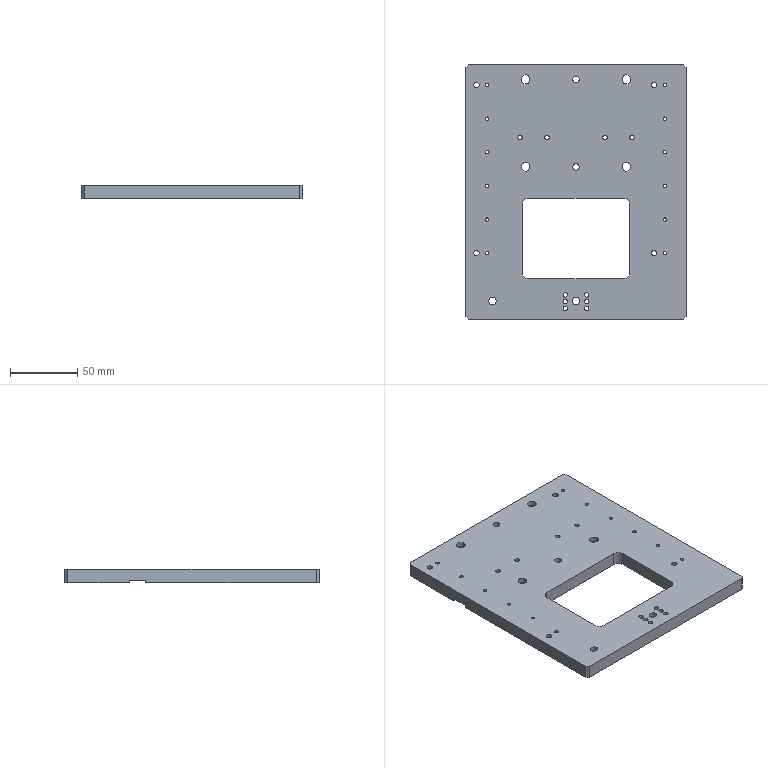Part | 1 solid | 68 faces | box 164 x 189 x 10 mm | volume 251895 mm3 | cylinder 44 | plane 24 | commonest cylinder face diameters 2.5 x12 3.3 x10 10 x6 4 x4 6.6 x4 11 x4